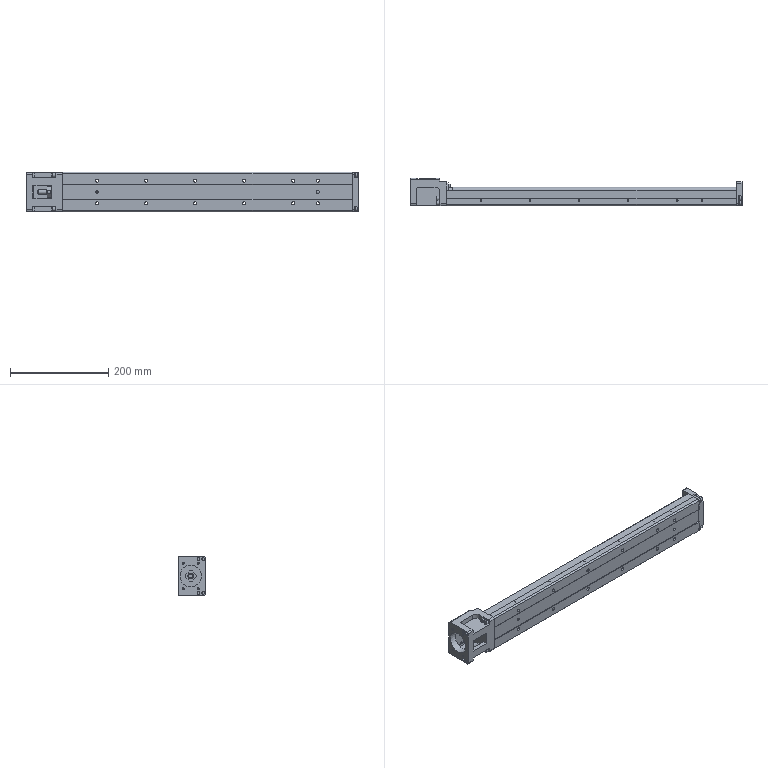Part | STEP file | LX4520CP-MX-B1-A4560-590-EP3_b | 1 solid | 385 faces | box 677 x 56 x 80 mm | volume 1131929 mm3 | plane 232 | cylinder 117 | cone 35 | torus 1 | commonest cylinder face diameters 6 x14 2.459 x12 6.6 x12 11 x12 8.3 x8 8.5 x8